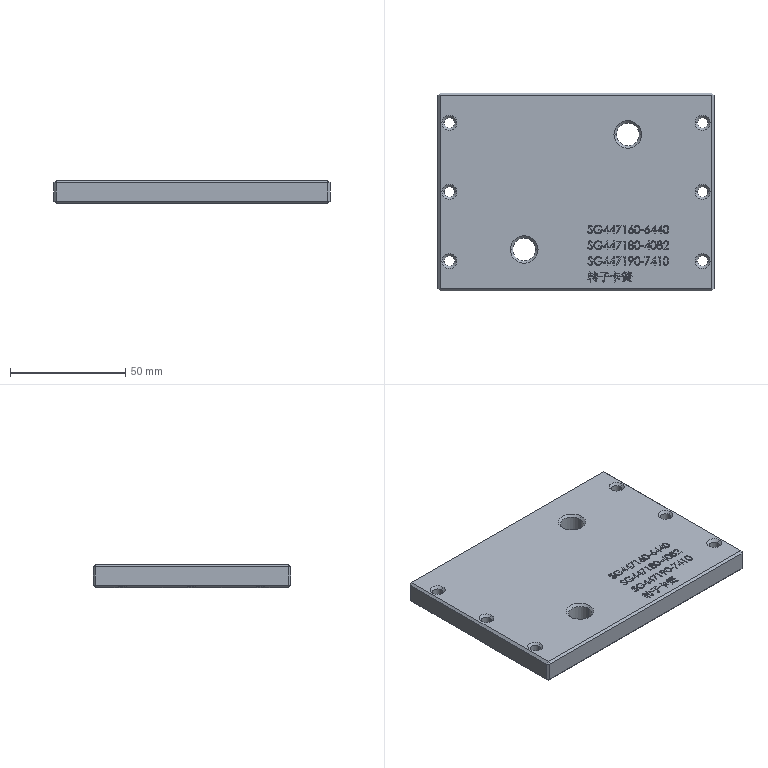Part | STEP file | Base-10P30 rotor clip | 1 solid | 802 faces | box 120 x 86 x 10 mm | volume 99024 mm3 | plane 506 | spline 236 | cone 32 | cylinder 28 | commonest cylinder face diameters 4.5 x12 8 x12 10 x4